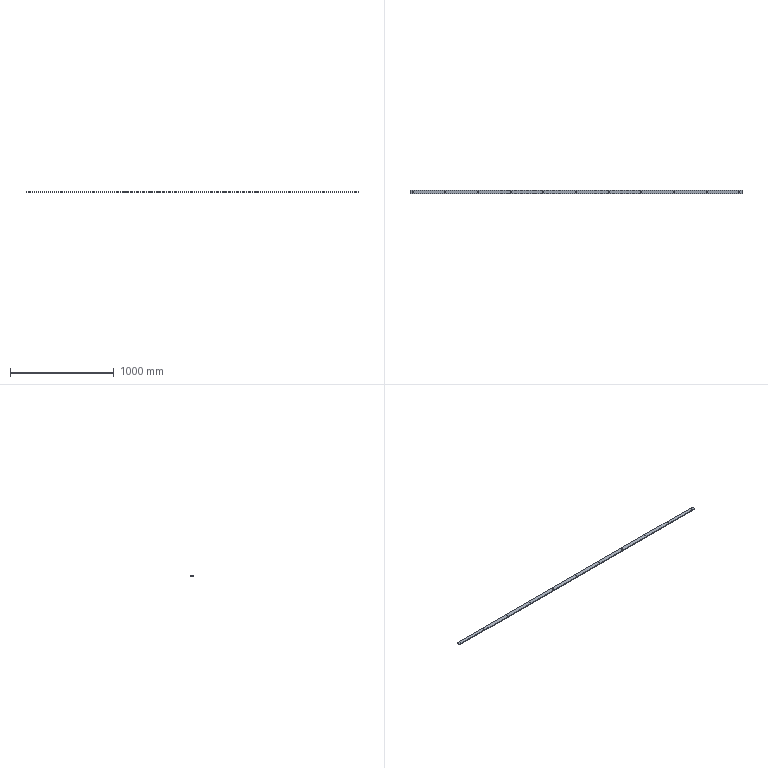Part | SolidWorks | features FlatPattern 1, HoleWzd 1, SMBaseFlange 1, SheetMetal 1 | 1 solid | 28 faces | box 3200 x 35 x 8 mm | volume 891006 mm3 | cylinder 22 | plane 6 | commonest cylinder face diameters 8.5 x22
STEP:
#1=CARTESIAN_POINT('',(-1579.25,0.,-8.));
#2=VERTEX_POINT('',#1);
#3=CARTESIAN_POINT('',(-1570.75,0.,-8.));
#4=VERTEX_POINT('',#3);
#5=CARTESIAN_POINT('',(-1575.,0.,-8.));
#6=DIRECTION('',(0.,0.,1.));
#7=DIRECTION('',(1.,0.,0.));
#8=AXIS2_PLACEMENT_3D('',#5,#6,#7);
#9=CIRCLE('',#8,4.25);
#10=EDGE_CURVE('',#2,#4,#9,.T.);
#11=ORIENTED_EDGE('',*,*,#10,.F.);
#12=CARTESIAN_POINT('',(-1579.25,0.,0.));
#13=VERTEX_POINT('',#12);
#14=CARTESIAN_POINT('',(-1579.25,0.,0.));
#15=DIRECTION('',(0.,0.,1.));
#16=VECTOR('',#15,1000.);
#17=LINE('',#14,#16);
#18=EDGE_CURVE('',#2,#13,#17,.T.);
#19=ORIENTED_EDGE('',*,*,#18,.T.);
#20=CARTESIAN_POINT('',(-1570.75,0.,0.));
#21=VERTEX_POINT('',#20);
#22=CARTESIAN_POINT('',(-1575.,0.,0.));
#23=DIRECTION('',(0.,0.,1.));
#24=DIRECTION('',(1.,0.,0.));
#25=AXIS2_PLACEMENT_3D('',#22,#23,#24);
#26=CIRCLE('',#25,4.25);
#27=EDGE_CURVE('',#13,#21,#26,.T.);
#28=ORIENTED_EDGE('',*,*,#27,.T.);
#29=CARTESIAN_POINT('',(-1570.75,0.,0.));
#30=DIRECTION('',(0.,0.,1.));
#31=VECTOR('',#30,1000.);
#32=LINE('',#29,#31);
#33=EDGE_CURVE('',#4,#21,#32,.T.);
#34=ORIENTED_EDGE('',*,*,#33,.F.);
#35=EDGE_LOOP('',(#11,#19,#28,#34));
#36=FACE_OUTER_BOUND('',#35,.T.);
#37=CARTESIAN_POINT('',(-1575.,0.,0.));
#38=DIRECTION('',(0.,0.,1.));
#39=DIRECTION('',(1.,0.,0.));
#40=AXIS2_PLACEMENT_3D('',#37,#38,#39);
#41=CYLINDRICAL_SURFACE('',#40,4.25);
#42=ADVANCED_FACE('',(#36),#41,.F.);
#43=CARTESIAN_POINT('',(-1264.25,0.,-8.));
#44=VERTEX_POINT('',#43);
#45=CARTESIAN_POINT('',(-1255.75,0.,-8.));
#46=VERTEX_POINT('',#45);
#47=CARTESIAN_POINT('',(-1260.,0.,-8.));
#48=DIRECTION('',(0.,0.,1.));
#49=DIRECTION('',(1.,0.,0.));
#50=AXIS2_PLACEMENT_3D('',#47,#48,#49);
#51=CIRCLE('',#50,4.25);
#52=EDGE_CURVE('',#44,#46,#51,.T.);
#53=ORIENTED_EDGE('',*,*,#52,.F.);
#54=CARTESIAN_POINT('',(-1264.25,0.,0.));
#55=VERTEX_POINT('',#54);
#56=CARTESIAN_POINT('',(-1264.25,0.,0.));
#57=DIRECTION('',(0.,0.,1.));
#58=VECTOR('',#57,1000.);
#59=LINE('',#56,#58);
#60=EDGE_CURVE('',#44,#55,#59,.T.);
#61=ORIENTED_EDGE('',*,*,#60,.T.);
#62=CARTESIAN_POINT('',(-1255.75,0.,0.));
#63=VERTEX_POINT('',#62);
#64=CARTESIAN_POINT('',(-1260.,0.,0.));
#65=DIRECTION('',(0.,0.,1.));
#66=DIRECTION('',(1.,0.,0.));
#67=AXIS2_PLACEMENT_3D('',#64,#65,#66);
#68=CIRCLE('',#67,4.25);
#69=EDGE_CURVE('',#55,#63,#68,.T.);
#70=ORIENTED_EDGE('',*,*,#69,.T.);
#71=CARTESIAN_POINT('',(-1255.75,0.,0.));
#72=DIRECTION('',(0.,0.,1.));
#73=VECTOR('',#72,1000.);
#74=LINE('',#71,#73);
#75=EDGE_CURVE('',#46,#63,#74,.T.);
#76=ORIENTED_EDGE('',*,*,#75,.F.);
#77=EDGE_LOOP('',(#53,#61,#70,#76));
#78=FACE_OUTER_BOUND('',#77,.T.);
#79=CARTESIAN_POINT('',(-1260.,0.,0.));
#80=DIRECTION('',(0.,0.,1.));
#81=DIRECTION('',(1.,0.,0.));
#82=AXIS2_PLACEMENT_3D('',#79,#80,#81);
#83=CYLINDRICAL_SURFACE('',#82,4.25);
#84=ADVANCED_FACE('',(#78),#83,.F.);
#85=CARTESIAN_POINT('',(-949.25,0.,-8.));
#86=VERTEX_POINT('',#85);
#87=CARTESIAN_POINT('',(-940.75,0.,-8.));
#88=VERTEX_POINT('',#87);
#89=CARTESIAN_POINT('',(-945.,0.,-8.));
#90=DIRECTION('',(0.,0.,1.));
#91=DIRECTION('',(1.,0.,0.));
#92=AXIS2_PLACEMENT_3D('',#89,#90,#91);
#93=CIRCLE('',#92,4.25);
#94=EDGE_CURVE('',#86,#88,#93,.T.);
#95=ORIENTED_EDGE('',*,*,#94,.F.);
#96=CARTESIAN_POINT('',(-949.25,0.,0.));
#97=VERTEX_POINT('',#96);
#98=CARTESIAN_POINT('',(-949.25,0.,0.));
#99=DIRECTION('',(0.,0.,1.));
#100=VECTOR('',#99,1000.);
#101=LINE('',#98,#100);
#102=EDGE_CURVE('',#86,#97,#101,.T.);
#103=ORIENTED_EDGE('',*,*,#102,.T.);
#104=CARTESIAN_POINT('',(-940.75,0.,0.));
#105=VERTEX_POINT('',#104);
#106=CARTESIAN_POINT('',(-945.,0.,0.));
#107=DIRECTION('',(0.,0.,1.));
#108=DIRECTION('',(1.,0.,0.));
#109=AXIS2_PLACEMENT_3D('',#106,#107,#108);
#110=CIRCLE('',#109,4.25);
#111=EDGE_CURVE('',#97,#105,#110,.T.);
#112=ORIENTED_EDGE('',*,*,#111,.T.);
#113=CARTESIAN_POINT('',(-940.75,0.,0.));
#114=DIRECTION('',(0.,0.,1.));
#115=VECTOR('',#114,1000.);
#116=LINE('',#113,#115);
#117=EDGE_CURVE('',#88,#105,#116,.T.);
#118=ORIENTED_EDGE('',*,*,#117,.F.);
#119=EDGE_LOOP('',(#95,#103,#112,#118));
#120=FACE_OUTER_BOUND('',#119,.T.);
#121=CARTESIAN_POINT('',(-945.,0.,0.));
#122=DIRECTION('',(0.,0.,1.));
#123=DIRECTION('',(1.,0.,0.));
#124=AXIS2_PLACEMENT_3D('',#121,#122,#123);
#125=CYLINDRICAL_SURFACE('',#124,4.25);
#126=ADVANCED_FACE('',(#120),#125,.F.);
#127=CARTESIAN_POINT('',(-634.25,0.,-8.));
#128=VERTEX_POINT('',#127);
#129=CARTESIAN_POINT('',(-625.75,0.,-8.));
#130=VERTEX_POINT('',#129);
#131=CARTESIAN_POINT('',(-630.,0.,-8.));
#132=DIRECTION('',(0.,0.,1.));
#133=DIRECTION('',(1.,0.,0.));
#134=AXIS2_PLACEMENT_3D('',#131,#132,#133);
#135=CIRCLE('',#134,4.25);
#136=EDGE_CURVE('',#128,#130,#135,.T.);
#137=ORIENTED_EDGE('',*,*,#136,.F.);
#138=CARTESIAN_POINT('',(-634.25,0.,0.));
#139=VERTEX_POINT('',#138);
#140=CARTESIAN_POINT('',(-634.25,0.,0.));
#141=DIRECTION('',(0.,0.,1.));
#142=VECTOR('',#141,1000.);
#143=LINE('',#140,#142);
#144=EDGE_CURVE('',#128,#139,#143,.T.);
#145=ORIENTED_EDGE('',*,*,#144,.T.);
#146=CARTESIAN_POINT('',(-625.75,0.,0.));
#147=VERTEX_POINT('',#146);
#148=CARTESIAN_POINT('',(-630.,0.,0.));
#149=DIRECTION('',(0.,0.,1.));
#150=DIRECTION('',(1.,0.,0.));
#151=AXIS2_PLACEMENT_3D('',#148,#149,#150);
#152=CIRCLE('',#151,4.25);
#153=EDGE_CURVE('',#139,#147,#152,.T.);
#154=ORIENTED_EDGE('',*,*,#153,.T.);
#155=CARTESIAN_POINT('',(-625.75,0.,0.));
#156=DIRECTION('',(0.,0.,1.));
#157=VECTOR('',#156,1000.);
#158=LINE('',#155,#157);
#159=EDGE_CURVE('',#130,#147,#158,.T.);
#160=ORIENTED_EDGE('',*,*,#159,.F.);
#161=EDGE_LOOP('',(#137,#145,#154,#160));
#162=FACE_OUTER_BOUND('',#161,.T.);
#163=CARTESIAN_POINT('',(-630.,0.,0.));
#164=DIRECTION('',(0.,0.,1.));
#165=DIRECTION('',(1.,0.,0.));
#166=AXIS2_PLACEMENT_3D('',#163,#164,#165);
#167=CYLINDRICAL_SURFACE('',#166,4.25);
#168=ADVANCED_FACE('',(#162),#167,.F.);
#169=CARTESIAN_POINT('',(-319.25,0.,-8.));
#170=VERTEX_POINT('',#169);
#171=CARTESIAN_POINT('',(-310.75,0.,-8.));
#172=VERTEX_POINT('',#171);
#173=CARTESIAN_POINT('',(-315.,0.,-8.));
#174=DIRECTION('',(0.,0.,1.));
#175=DIRECTION('',(1.,0.,0.));
#176=AXIS2_PLACEMENT_3D('',#173,#174,#175);
#177=CIRCLE('',#176,4.25);
#178=EDGE_CURVE('',#170,#172,#177,.T.);
#179=ORIENTED_EDGE('',*,*,#178,.F.);
#180=CARTESIAN_POINT('',(-319.25,0.,0.));
#181=VERTEX_POINT('',#180);
#182=CARTESIAN_POINT('',(-319.25,0.,0.));
#183=DIRECTION('',(0.,0.,1.));
#184=VECTOR('',#183,1000.);
#185=LINE('',#182,#184);
#186=EDGE_CURVE('',#170,#181,#185,.T.);
#187=ORIENTED_EDGE('',*,*,#186,.T.);
#188=CARTESIAN_POINT('',(-310.75,0.,0.));
#189=VERTEX_POINT('',#188);
#190=CARTESIAN_POINT('',(-315.,0.,0.));
#191=DIRECTION('',(0.,0.,1.));
#192=DIRECTION('',(1.,0.,0.));
#193=AXIS2_PLACEMENT_3D('',#190,#191,#192);
#194=CIRCLE('',#193,4.25);
#195=EDGE_CURVE('',#181,#189,#194,.T.);
#196=ORIENTED_EDGE('',*,*,#195,.T.);
#197=CARTESIAN_POINT('',(-310.75,0.,0.));
#198=DIRECTION('',(0.,0.,1.));
#199=VECTOR('',#198,1000.);
#200=LINE('',#197,#199);
#201=EDGE_CURVE('',#172,#189,#200,.T.);
#202=ORIENTED_EDGE('',*,*,#201,.F.);
#203=EDGE_LOOP('',(#179,#187,#196,#202));
#204=FACE_OUTER_BOUND('',#203,.T.);
#205=CARTESIAN_POINT('',(-315.,0.,0.));
#206=DIRECTION('',(0.,0.,1.));
#207=DIRECTION('',(1.,0.,0.));
#208=AXIS2_PLACEMENT_3D('',#205,#206,#207);
#209=CYLINDRICAL_SURFACE('',#208,4.25);
#210=ADVANCED_FACE('',(#204),#209,.F.);
#211=CARTESIAN_POINT('',(-4.25,0.,-8.));
#212=VERTEX_POINT('',#211);
#213=CARTESIAN_POINT('',(4.25,0.,-8.));
#214=VERTEX_POINT('',#213);
#215=CARTESIAN_POINT('',(0.,0.,-8.));
#216=DIRECTION('',(0.,0.,1.));
#217=DIRECTION('',(1.,0.,0.));
#218=AXIS2_PLACEMENT_3D('',#215,#216,#217);
#219=CIRCLE('',#218,4.25);
#220=EDGE_CURVE('',#212,#214,#219,.T.);
#221=ORIENTED_EDGE('',*,*,#220,.F.);
#222=CARTESIAN_POINT('',(-4.25,0.,0.));
#223=VERTEX_POINT('',#222);
#224=CARTESIAN_POINT('',(-4.25,0.,0.));
#225=DIRECTION('',(0.,0.,1.));
#226=VECTOR('',#225,1000.);
#227=LINE('',#224,#226);
#228=EDGE_CURVE('',#212,#223,#227,.T.);
#229=ORIENTED_EDGE('',*,*,#228,.T.);
#230=CARTESIAN_POINT('',(4.25,0.,0.));
#231=VERTEX_POINT('',#230);
#232=CARTESIAN_POINT('',(0.,0.,0.));
#233=DIRECTION('',(0.,0.,1.));
#234=DIRECTION('',(1.,0.,0.));
#235=AXIS2_PLACEMENT_3D('',#232,#233,#234);
#236=CIRCLE('',#235,4.25);
#237=EDGE_CURVE('',#223,#231,#236,.T.);
#238=ORIENTED_EDGE('',*,*,#237,.T.);
#239=CARTESIAN_POINT('',(4.25,0.,0.));
#240=DIRECTION('',(0.,0.,1.));
#241=VECTOR('',#240,1000.);
#242=LINE('',#239,#241);
#243=EDGE_CURVE('',#214,#231,#242,.T.);
#244=ORIENTED_EDGE('',*,*,#243,.F.);
#245=EDGE_LOOP('',(#221,#229,#238,#244));
#246=FACE_OUTER_BOUND('',#245,.T.);
#247=CARTESIAN_POINT('',(0.,0.,0.));
#248=DIRECTION('',(0.,0.,1.));
#249=DIRECTION('',(1.,0.,0.));
#250=AXIS2_PLACEMENT_3D('',#247,#248,#249);
#251=CYLINDRICAL_SURFACE('',#250,4.25);
#252=ADVANCED_FACE('',(#246),#251,.F.);
#253=CARTESIAN_POINT('',(310.75,0.,-8.));
#254=VERTEX_POINT('',#253);
#255=CARTESIAN_POINT('',(319.25,0.,-8.));
#256=VERTEX_POINT('',#255);
#257=CARTESIAN_POINT('',(315.,0.,-8.));
#258=DIRECTION('',(0.,0.,1.));
#259=DIRECTION('',(1.,0.,0.));
#260=AXIS2_PLACEMENT_3D('',#257,#258,#259);
#261=CIRCLE('',#260,4.25);
#262=EDGE_CURVE('',#254,#256,#261,.T.);
#263=ORIENTED_EDGE('',*,*,#262,.F.);
#264=CARTESIAN_POINT('',(310.75,0.,0.));
#265=VERTEX_POINT('',#264);
#266=CARTESIAN_POINT('',(310.75,0.,0.));
#267=DIRECTION('',(0.,0.,1.));
#268=VECTOR('',#267,1000.);
#269=LINE('',#266,#268);
#270=EDGE_CURVE('',#254,#265,#269,.T.);
#271=ORIENTED_EDGE('',*,*,#270,.T.);
#272=CARTESIAN_POINT('',(319.25,0.,0.));
#273=VERTEX_POINT('',#272);
#274=CARTESIAN_POINT('',(315.,0.,0.));
#275=DIRECTION('',(0.,0.,1.));
#276=DIRECTION('',(1.,0.,0.));
#277=AXIS2_PLACEMENT_3D('',#274,#275,#276);
#278=CIRCLE('',#277,4.25);
#279=EDGE_CURVE('',#265,#273,#278,.T.);
#280=ORIENTED_EDGE('',*,*,#279,.T.);
#281=CARTESIAN_POINT('',(319.25,0.,0.));
#282=DIRECTION('',(0.,0.,1.));
#283=VECTOR('',#282,1000.);
#284=LINE('',#281,#283);
#285=EDGE_CURVE('',#256,#273,#284,.T.);
#286=ORIENTED_EDGE('',*,*,#285,.F.);
#287=EDGE_LOOP('',(#263,#271,#280,#286));
#288=FACE_OUTER_BOUND('',#287,.T.);
#289=CARTESIAN_POINT('',(315.,0.,0.));
#290=DIRECTION('',(0.,0.,1.));
#291=DIRECTION('',(1.,0.,0.));
#292=AXIS2_PLACEMENT_3D('',#289,#290,#291);
#293=CYLINDRICAL_SURFACE('',#292,4.25);
#294=ADVANCED_FACE('',(#288),#293,.F.);
#295=CARTESIAN_POINT('',(625.75,0.,-8.));
#296=VERTEX_POINT('',#295);
#297=CARTESIAN_POINT('',(634.25,0.,-8.));
#298=VERTEX_POINT('',#297);
#299=CARTESIAN_POINT('',(630.,0.,-8.));
#300=DIRECTION('',(0.,0.,1.));
#301=DIRECTION('',(1.,0.,0.));
#302=AXIS2_PLACEMENT_3D('',#299,#300,#301);
#303=CIRCLE('',#302,4.25);
#304=EDGE_CURVE('',#296,#298,#303,.T.);
#305=ORIENTED_EDGE('',*,*,#304,.F.);
#306=CARTESIAN_POINT('',(625.75,0.,0.));
#307=VERTEX_POINT('',#306);
#308=CARTESIAN_POINT('',(625.75,0.,0.));
#309=DIRECTION('',(0.,0.,1.));
#310=VECTOR('',#309,1000.);
#311=LINE('',#308,#310);
#312=EDGE_CURVE('',#296,#307,#311,.T.);
#313=ORIENTED_EDGE('',*,*,#312,.T.);
#314=CARTESIAN_POINT('',(634.25,0.,0.));
#315=VERTEX_POINT('',#314);
#316=CARTESIAN_POINT('',(630.,0.,0.));
#317=DIRECTION('',(0.,0.,1.));
#318=DIRECTION('',(1.,0.,0.));
#319=AXIS2_PLACEMENT_3D('',#316,#317,#318);
#320=CIRCLE('',#319,4.25);
#321=EDGE_CURVE('',#307,#315,#320,.T.);
#322=ORIENTED_EDGE('',*,*,#321,.T.);
#323=CARTESIAN_POINT('',(634.25,0.,0.));
#324=DIRECTION('',(0.,0.,1.));
#325=VECTOR('',#324,1000.);
#326=LINE('',#323,#325);
#327=EDGE_CURVE('',#298,#315,#326,.T.);
#328=ORIENTED_EDGE('',*,*,#327,.F.);
#329=EDGE_LOOP('',(#305,#313,#322,#328));
#330=FACE_OUTER_BOUND('',#329,.T.);
#331=CARTESIAN_POINT('',(630.,0.,0.));
#332=DIRECTION('',(0.,0.,1.));
#333=DIRECTION('',(1.,0.,0.));
#334=AXIS2_PLACEMENT_3D('',#331,#332,#333);
#335=CYLINDRICAL_SURFACE('',#334,4.25);
#336=ADVANCED_FACE('',(#330),#335,.F.);
#337=CARTESIAN_POINT('',(940.75,0.,-8.));
#338=VERTEX_POINT('',#337);
#339=CARTESIAN_POINT('',(949.25,0.,-8.));
#340=VERTEX_POINT('',#339);
#341=CARTESIAN_POINT('',(945.,0.,-8.));
#342=DIRECTION('',(0.,0.,1.));
#343=DIRECTION('',(1.,0.,0.));
#344=AXIS2_PLACEMENT_3D('',#341,#342,#343);
#345=CIRCLE('',#344,4.25);
#346=EDGE_CURVE('',#338,#340,#345,.T.);
#347=ORIENTED_EDGE('',*,*,#346,.F.);
#348=CARTESIAN_POINT('',(940.75,0.,0.));
#349=VERTEX_POINT('',#348);
#350=CARTESIAN_POINT('',(940.75,0.,0.));
#351=DIRECTION('',(0.,0.,1.));
#352=VECTOR('',#351,1000.);
#353=LINE('',#350,#352);
#354=EDGE_CURVE('',#338,#349,#353,.T.);
#355=ORIENTED_EDGE('',*,*,#354,.T.);
#356=CARTESIAN_POINT('',(949.25,0.,0.));
#357=VERTEX_POINT('',#356);
#358=CARTESIAN_POINT('',(945.,0.,0.));
#359=DIRECTION('',(0.,0.,1.));
#360=DIRECTION('',(1.,0.,0.));
#361=AXIS2_PLACEMENT_3D('',#358,#359,#360);
#362=CIRCLE('',#361,4.25);
#363=EDGE_CURVE('',#349,#357,#362,.T.);
#364=ORIENTED_EDGE('',*,*,#363,.T.);
#365=CARTESIAN_POINT('',(949.25,0.,0.));
#366=DIRECTION('',(0.,0.,1.));
#367=VECTOR('',#366,1000.);
#368=LINE('',#365,#367);
#369=EDGE_CURVE('',#340,#357,#368,.T.);
#370=ORIENTED_EDGE('',*,*,#369,.F.);
#371=EDGE_LOOP('',(#347,#355,#364,#370));
#372=FACE_OUTER_BOUND('',#371,.T.);
#373=CARTESIAN_POINT('',(945.,0.,0.));
#374=DIRECTION('',(0.,0.,1.));
#375=DIRECTION('',(1.,0.,0.));
#376=AXIS2_PLACEMENT_3D('',#373,#374,#375);
#377=CYLINDRICAL_SURFACE('',#376,4.25);
#378=ADVANCED_FACE('',(#372),#377,.F.);
#379=CARTESIAN_POINT('',(1255.75,0.,-8.));
#380=VERTEX_POINT('',#379);
#381=CARTESIAN_POINT('',(1264.25,0.,-8.));
#382=VERTEX_POINT('',#381);
#383=CARTESIAN_POINT('',(1260.,0.,-8.));
#384=DIRECTION('',(0.,0.,1.));
#385=DIRECTION('',(1.,0.,0.));
#386=AXIS2_PLACEMENT_3D('',#383,#384,#385);
#387=CIRCLE('',#386,4.25);
#388=EDGE_CURVE('',#380,#382,#387,.T.);
#389=ORIENTED_EDGE('',*,*,#388,.F.);
#390=CARTESIAN_POINT('',(1255.75,0.,0.));
#391=VERTEX_POINT('',#390);
#392=CARTESIAN_POINT('',(1255.75,0.,0.));
#393=DIRECTION('',(0.,0.,1.));
#394=VECTOR('',#393,1000.);
#395=LINE('',#392,#394);
#396=EDGE_CURVE('',#380,#391,#395,.T.);
#397=ORIENTED_EDGE('',*,*,#396,.T.);
#398=CARTESIAN_POINT('',(1264.25,0.,0.));
#399=VERTEX_POINT('',#398);
#400=CARTESIAN_POINT('',(1260.,0.,0.));
#401=DIRECTION('',(0.,0.,1.));
#402=DIRECTION('',(1.,0.,0.));
#403=AXIS2_PLACEMENT_3D('',#400,#401,#402);
#404=CIRCLE('',#403,4.25);
#405=EDGE_CURVE('',#391,#399,#404,.T.);
#406=ORIENTED_EDGE('',*,*,#405,.T.);
#407=CARTESIAN_POINT('',(1264.25,0.,0.));
#408=DIRECTION('',(0.,0.,1.));
#409=VECTOR('',#408,1000.);
#410=LINE('',#407,#409);
#411=EDGE_CURVE('',#382,#399,#410,.T.);
#412=ORIENTED_EDGE('',*,*,#411,.F.);
#413=EDGE_LOOP('',(#389,#397,#406,#412));
#414=FACE_OUTER_BOUND('',#413,.T.);
#415=CARTESIAN_POINT('',(1260.,0.,0.));
#416=DIRECTION('',(0.,0.,1.));
#417=DIRECTION('',(1.,0.,0.));
#418=AXIS2_PLACEMENT_3D('',#415,#416,#417);
#419=CYLINDRICAL_SURFACE('',#418,4.25);
#420=ADVANCED_FACE('',(#414),#419,.F.);
#421=CARTESIAN_POINT('',(1570.75,0.,-8.));
#422=VERTEX_POINT('',#421);
#423=CARTESIAN_POINT('',(1579.25,0.,-8.));
#424=VERTEX_POINT('',#423);
#425=CARTESIAN_POINT('',(1575.,0.,-8.));
#426=DIRECTION('',(0.,0.,1.));
#427=DIRECTION('',(1.,0.,0.));
#428=AXIS2_PLACEMENT_3D('',#425,#426,#427);
#429=CIRCLE('',#428,4.25);
#430=EDGE_CURVE('',#422,#424,#429,.T.);
#431=ORIENTED_EDGE('',*,*,#430,.F.);
#432=CARTESIAN_POINT('',(1570.75,0.,0.));
#433=VERTEX_POINT('',#432);
#434=CARTESIAN_POINT('',(1570.75,0.,0.));
#435=DIRECTION('',(0.,0.,1.));
#436=VECTOR('',#435,1000.);
#437=LINE('',#434,#436);
#438=EDGE_CURVE('',#422,#433,#437,.T.);
#439=ORIENTED_EDGE('',*,*,#438,.T.);
#440=CARTESIAN_POINT('',(1579.25,0.,0.));
#441=VERTEX_POINT('',#440);
#442=CARTESIAN_POINT('',(1575.,0.,0.));
#443=DIRECTION('',(0.,0.,1.));
#444=DIRECTION('',(1.,0.,0.));
#445=AXIS2_PLACEMENT_3D('',#442,#443,#444);
#446=CIRCLE('',#445,4.25);
#447=EDGE_CURVE('',#433,#441,#446,.T.);
#448=ORIENTED_EDGE('',*,*,#447,.T.);
#449=CARTESIAN_POINT('',(1579.25,0.,0.));
#450=DIRECTION('',(0.,0.,1.));
#451=VECTOR('',#450,1000.);
#452=LINE('',#449,#451);
#453=EDGE_CURVE('',#424,#441,#452,.T.);
#454=ORIENTED_EDGE('',*,*,#453,.F.);
#455=EDGE_LOOP('',(#431,#439,#448,#454));
#456=FACE_OUTER_BOUND('',#455,.T.);
#457=CARTESIAN_POINT('',(1575.,0.,0.));
#458=DIRECTION('',(0.,0.,1.));
#459=DIRECTION('',(1.,0.,0.));
#460=AXIS2_PLACEMENT_3D('',#457,#458,#459);
#461=CYLINDRICAL_SURFACE('',#460,4.25);
#462=ADVANCED_FACE('',(#456),#461,.F.);
#463=CARTESIAN_POINT('',(1600.,-17.5,0.));
#464=VERTEX_POINT('',#463);
#465=CARTESIAN_POINT('',(1600.,17.5,0.));
#466=VERTEX_POINT('',#465);
#467=CARTESIAN_POINT('',(1600.,17.5,0.));
#468=DIRECTION('',(0.,1.,0.));
#469=VECTOR('',#468,1000.);
#470=LINE('',#467,#469);
#471=EDGE_CURVE('',#464,#466,#470,.T.);
#472=ORIENTED_EDGE('',*,*,#471,.F.);
#473=CARTESIAN_POINT('',(1600.,-17.5,-8.));
#474=VERTEX_POINT('',#473);
#475=CARTESIAN_POINT('',(1600.,-17.5,-8.));
#476=DIRECTION('',(0.,0.,1.));
#477=VECTOR('',#476,1000.);
#478=LINE('',#475,#477);
#479=EDGE_CURVE('',#474,#464,#478,.T.);
#480=ORIENTED_EDGE('',*,*,#479,.F.);
#481=CARTESIAN_POINT('',(1600.,17.5,-8.));
#482=VERTEX_POINT('',#481);
#483=CARTESIAN_POINT('',(1600.,17.5,-8.));
#484=DIRECTION('',(0.,1.,0.));
#485=VECTOR('',#484,1000.);
#486=LINE('',#483,#485);
#487=EDGE_CURVE('',#474,#482,#486,.T.);
#488=ORIENTED_EDGE('',*,*,#487,.T.);
#489=CARTESIAN_POINT('',(1600.,17.5,-8.));
#490=DIRECTION('',(0.,0.,1.));
#491=VECTOR('',#490,1000.);
#492=LINE('',#489,#491);
#493=EDGE_CURVE('',#482,#466,#492,.T.);
#494=ORIENTED_EDGE('',*,*,#493,.T.);
#495=EDGE_LOOP('',(#472,#480,#488,#494));
#496=FACE_OUTER_BOUND('',#495,.T.);
#497=CARTESIAN_POINT('',(1600.,17.5,-8.));
#498=DIRECTION('',(1.,0.,0.));
#499=DIRECTION('',(0.,0.,-1.));
#500=AXIS2_PLACEMENT_3D('',#497,#498,#499);
#501=PLANE('',#500);
#502=ADVANCED_FACE('',(#496),#501,.T.);
#503=CARTESIAN_POINT('',(-1600.,-17.5,0.));
#504=VERTEX_POINT('',#503);
#505=CARTESIAN_POINT('',(-1600.,-17.5,0.));
#506=DIRECTION('',(1.,0.,0.));
#507=VECTOR('',#506,1000.);
#508=LINE('',#505,#507);
#509=EDGE_CURVE('',#504,#464,#508,.T.);
#510=ORIENTED_EDGE('',*,*,#509,.F.);
#511=CARTESIAN_POINT('',(-1600.,-17.5,-8.));
#512=VERTEX_POINT('',#511);
#513=CARTESIAN_POINT('',(-1600.,-17.5,-8.));
#514=DIRECTION('',(0.,0.,1.));
#515=VECTOR('',#514,1000.);
#516=LINE('',#513,#515);
#517=EDGE_CURVE('',#512,#504,#516,.T.);
#518=ORIENTED_EDGE('',*,*,#517,.F.);
#519=CARTESIAN_POINT('',(-1600.,-17.5,-8.));
#520=DIRECTION('',(1.,0.,0.));
#521=VECTOR('',#520,1000.);
#522=LINE('',#519,#521);
#523=EDGE_CURVE('',#512,#474,#522,.T.);
#524=ORIENTED_EDGE('',*,*,#523,.T.);
#525=ORIENTED_EDGE('',*,*,#479,.T.);
#526=EDGE_LOOP('',(#510,#518,#524,#525));
#527=FACE_OUTER_BOUND('',#526,.T.);
#528=CARTESIAN_POINT('',(-1600.,-17.5,-8.));
#529=DIRECTION('',(0.,-1.,0.));
#530=DIRECTION('',(0.,0.,-1.));
#531=AXIS2_PLACEMENT_3D('',#528,#529,#530);
#532=PLANE('',#531);
#533=ADVANCED_FACE('',(#527),#532,.T.);
#534=CARTESIAN_POINT('',(-1600.,17.5,0.));
#535=VERTEX_POINT('',#534);
#536=CARTESIAN_POINT('',(-1600.,17.5,0.));
#537=DIRECTION('',(0.,-1.,0.));
#538=VECTOR('',#537,1000.);
#539=LINE('',#536,#538);
#540=EDGE_CURVE('',#535,#504,#539,.T.);
#541=ORIENTED_EDGE('',*,*,#540,.F.);
#542=CARTESIAN_POINT('',(-1600.,17.5,-8.));
#543=VERTEX_POINT('',#542);
#544=CARTESIAN_POINT('',(-1600.,17.5,-8.));
#545=DIRECTION('',(0.,0.,1.));
#546=VECTOR('',#545,1000.);
#547=LINE('',#544,#546);
#548=EDGE_CURVE('',#543,#535,#547,.T.);
#549=ORIENTED_EDGE('',*,*,#548,.F.);
#550=CARTESIAN_POINT('',(-1600.,17.5,-8.));
#551=DIRECTION('',(0.,-1.,0.));
#552=VECTOR('',#551,1000.);
#553=LINE('',#550,#552);
#554=EDGE_CURVE('',#543,#512,#553,.T.);
#555=ORIENTED_EDGE('',*,*,#554,.T.);
#556=ORIENTED_EDGE('',*,*,#517,.T.);
#557=EDGE_LOOP('',(#541,#549,#555,#556));
#558=FACE_OUTER_BOUND('',#557,.T.);
#559=CARTESIAN_POINT('',(-1600.,17.5,-8.));
#560=DIRECTION('',(-1.,0.,0.));
#561=DIRECTION('',(0.,0.,1.));
#562=AXIS2_PLACEMENT_3D('',#559,#560,#561);
#563=PLANE('',#562);
#564=ADVANCED_FACE('',(#558),#563,.T.);
#565=CARTESIAN_POINT('',(-1600.,17.5,0.));
#566=DIRECTION('',(-1.,0.,0.));
#567=VECTOR('',#566,1000.);
#568=LINE('',#565,#567);
#569=EDGE_CURVE('',#466,#535,#568,.T.);
#570=ORIENTED_EDGE('',*,*,#569,.F.);
#571=ORIENTED_EDGE('',*,*,#493,.F.);
#572=CARTESIAN_POINT('',(-1600.,17.5,-8.));
#573=DIRECTION('',(-1.,0.,0.));
#574=VECTOR('',#573,1000.);
#575=LINE('',#572,#574);
#576=EDGE_CURVE('',#482,#543,#575,.T.);
#577=ORIENTED_EDGE('',*,*,#576,.T.);
#578=ORIENTED_EDGE('',*,*,#548,.T.);
#579=EDGE_LOOP('',(#570,#571,#577,#578));
#580=FACE_OUTER_BOUND('',#579,.T.);
#581=CARTESIAN_POINT('',(-1600.,17.5,-8.));
#582=DIRECTION('',(0.,1.,0.));
#583=DIRECTION('',(0.,0.,1.));
#584=AXIS2_PLACEMENT_3D('',#581,#582,#583);
#585=PLANE('',#584);
#586=ADVANCED_FACE('',(#580),#585,.T.);
#587=CARTESIAN_POINT('',(-1575.,0.,-8.));
#588=DIRECTION('',(0.,0.,1.));
#589=DIRECTION('',(1.,0.,0.));
#590=AXIS2_PLACEMENT_3D('',#587,#588,#589);
#591=CIRCLE('',#590,4.25);
#592=EDGE_CURVE('',#4,#2,#591,.T.);
#593=ORIENTED_EDGE('',*,*,#592,.T.);
#594=ORIENTED_EDGE('',*,*,#10,.T.);
#595=EDGE_LOOP('',(#593,#594));
#596=FACE_BOUND('',#595,.T.);
#597=CARTESIAN_POINT('',(-1260.,0.,-8.));
#598=DIRECTION('',(0.,0.,1.));
#599=DIRECTION('',(1.,0.,0.));
#600=AXIS2_PLACEMENT_3D('',#597,#598,#599);
#601=CIRCLE('',#600,4.25);
#602=EDGE_CURVE('',#46,#44,#601,.T.);
#603=ORIENTED_EDGE('',*,*,#602,.T.);
#604=ORIENTED_EDGE('',*,*,#52,.T.);
#605=EDGE_LOOP('',(#603,#604));
#606=FACE_BOUND('',#605,.T.);
#607=CARTESIAN_POINT('',(-945.,0.,-8.));
#608=DIRECTION('',(0.,0.,1.));
#609=DIRECTION('',(1.,0.,0.));
#610=AXIS2_PLACEMENT_3D('',#607,#608,#609);
#611=CIRCLE('',#610,4.25);
#612=EDGE_CURVE('',#88,#86,#611,.T.);
#613=ORIENTED_EDGE('',*,*,#612,.T.);
#614=ORIENTED_EDGE('',*,*,#94,.T.);
#615=EDGE_LOOP('',(#613,#614));
#616=FACE_BOUND('',#615,.T.);
#617=CARTESIAN_POINT('',(-630.,0.,-8.));
#618=DIRECTION('',(0.,0.,1.));
#619=DIRECTION('',(1.,0.,0.));
#620=AXIS2_PLACEMENT_3D('',#617,#618,#619);
#621=CIRCLE('',#620,4.25);
#622=EDGE_CURVE('',#130,#128,#621,.T.);
#623=ORIENTED_EDGE('',*,*,#622,.T.);
#624=ORIENTED_EDGE('',*,*,#136,.T.);
#625=EDGE_LOOP('',(#623,#624));
#626=FACE_BOUND('',#625,.T.);
#627=CARTESIAN_POINT('',(-315.,0.,-8.));
#628=DIRECTION('',(0.,0.,1.));
#629=DIRECTION('',(1.,0.,0.));
#630=AXIS2_PLACEMENT_3D('',#627,#628,#629);
#631=CIRCLE('',#630,4.25);
#632=EDGE_CURVE('',#172,#170,#631,.T.);
#633=ORIENTED_EDGE('',*,*,#632,.T.);
#634=ORIENTED_EDGE('',*,*,#178,.T.);
#635=EDGE_LOOP('',(#633,#634));
#636=FACE_BOUND('',#635,.T.);
#637=CARTESIAN_POINT('',(0.,0.,-8.));
#638=DIRECTION('',(0.,0.,1.));
#639=DIRECTION('',(1.,0.,0.));
#640=AXIS2_PLACEMENT_3D('',#637,#638,#639);
#641=CIRCLE('',#640,4.25);
#642=EDGE_CURVE('',#214,#212,#641,.T.);
#643=ORIENTED_EDGE('',*,*,#642,.T.);
#644=ORIENTED_EDGE('',*,*,#220,.T.);
#645=EDGE_LOOP('',(#643,#644));
#646=FACE_BOUND('',#645,.T.);
#647=CARTESIAN_POINT('',(315.,0.,-8.));
#648=DIRECTION('',(0.,0.,1.));
#649=DIRECTION('',(1.,0.,0.));
#650=AXIS2_PLACEMENT_3D('',#647,#648,#649);
#651=CIRCLE('',#650,4.25);
#652=EDGE_CURVE('',#256,#254,#651,.T.);
#653=ORIENTED_EDGE('',*,*,#652,.T.);
#654=ORIENTED_EDGE('',*,*,#262,.T.);
#655=EDGE_LOOP('',(#653,#654));
#656=FACE_BOUND('',#655,.T.);
#657=CARTESIAN_POINT('',(630.,0.,-8.));
#658=DIRECTION('',(0.,0.,1.));
#659=DIRECTION('',(1.,0.,0.));
#660=AXIS2_PLACEMENT_3D('',#657,#658,#659);
#661=CIRCLE('',#660,4.25);
#662=EDGE_CURVE('',#298,#296,#661,.T.);
#663=ORIENTED_EDGE('',*,*,#662,.T.);
#664=ORIENTED_EDGE('',*,*,#304,.T.);
#665=EDGE_LOOP('',(#663,#664));
#666=FACE_BOUND('',#665,.T.);
#667=CARTESIAN_POINT('',(945.,0.,-8.));
#668=DIRECTION('',(0.,0.,1.));
#669=DIRECTION('',(1.,0.,0.));
#670=AXIS2_PLACEMENT_3D('',#667,#668,#669);
#671=CIRCLE('',#670,4.25);
#672=EDGE_CURVE('',#340,#338,#671,.T.);
#673=ORIENTED_EDGE('',*,*,#672,.T.);
#674=ORIENTED_EDGE('',*,*,#346,.T.);
#675=EDGE_LOOP('',(#673,#674));
#676=FACE_BOUND('',#675,.T.);
#677=CARTESIAN_POINT('',(1260.,0.,-8.));
#678=DIRECTION('',(0.,0.,1.));
#679=DIRECTION('',(1.,0.,0.));
#680=AXIS2_PLACEMENT_3D('',#677,#678,#679);
#681=CIRCLE('',#680,4.25);
#682=EDGE_CURVE('',#382,#380,#681,.T.);
#683=ORIENTED_EDGE('',*,*,#682,.T.);
#684=ORIENTED_EDGE('',*,*,#388,.T.);
#685=EDGE_LOOP('',(#683,#684));
#686=FACE_BOUND('',#685,.T.);
#687=CARTESIAN_POINT('',(1575.,0.,-8.));
#688=DIRECTION('',(0.,0.,1.));
#689=DIRECTION('',(1.,0.,0.));
#690=AXIS2_PLACEMENT_3D('',#687,#688,#689);
#691=CIRCLE('',#690,4.25);
#692=EDGE_CURVE('',#424,#422,#691,.T.);
#693=ORIENTED_EDGE('',*,*,#692,.T.);
#694=ORIENTED_EDGE('',*,*,#430,.T.);
#695=EDGE_LOOP('',(#693,#694));
#696=FACE_BOUND('',#695,.T.);
#697=ORIENTED_EDGE('',*,*,#487,.F.);
#698=ORIENTED_EDGE('',*,*,#523,.F.);
#699=ORIENTED_EDGE('',*,*,#554,.F.);
#700=ORIENTED_EDGE('',*,*,#576,.F.);
#701=EDGE_LOOP('',(#697,#698,#699,#700));
#702=FACE_OUTER_BOUND('',#701,.T.);
#703=CARTESIAN_POINT('',(0.,0.,-8.));
#704=DIRECTION('',(0.,0.,1.));
#705=DIRECTION('',(1.,0.,0.));
#706=AXIS2_PLACEMENT_3D('',#703,#704,#705);
#707=PLANE('',#706);
#708=ADVANCED_FACE('',(#596,#606,#616,#626,#636,#646,#656,#666,#676,#686,#696,#702),#707,.F.);
#709=CARTESIAN_POINT('',(-1575.,0.,0.));
#710=DIRECTION('',(0.,0.,1.));
#711=DIRECTION('',(1.,0.,0.));
#712=AXIS2_PLACEMENT_3D('',#709,#710,#711);
#713=CIRCLE('',#712,4.25);
#714=EDGE_CURVE('',#21,#13,#713,.T.);
#715=ORIENTED_EDGE('',*,*,#714,.F.);
#716=ORIENTED_EDGE('',*,*,#27,.F.);
#717=EDGE_LOOP('',(#715,#716));
#718=FACE_BOUND('',#717,.T.);
#719=CARTESIAN_POINT('',(-1260.,0.,0.));
#720=DIRECTION('',(0.,0.,1.));
#721=DIRECTION('',(1.,0.,0.));
#722=AXIS2_PLACEMENT_3D('',#719,#720,#721);
#723=CIRCLE('',#722,4.25);
#724=EDGE_CURVE('',#63,#55,#723,.T.);
#725=ORIENTED_EDGE('',*,*,#724,.F.);
#726=ORIENTED_EDGE('',*,*,#69,.F.);
#727=EDGE_LOOP('',(#725,#726));
#728=FACE_BOUND('',#727,.T.);
#729=CARTESIAN_POINT('',(-945.,0.,0.));
#730=DIRECTION('',(0.,0.,1.));
#731=DIRECTION('',(1.,0.,0.));
#732=AXIS2_PLACEMENT_3D('',#729,#730,#731);
#733=CIRCLE('',#732,4.25);
#734=EDGE_CURVE('',#105,#97,#733,.T.);
#735=ORIENTED_EDGE('',*,*,#734,.F.);
#736=ORIENTED_EDGE('',*,*,#111,.F.);
#737=EDGE_LOOP('',(#735,#736));
#738=FACE_BOUND('',#737,.T.);
#739=CARTESIAN_POINT('',(-630.,0.,0.));
#740=DIRECTION('',(0.,0.,1.));
#741=DIRECTION('',(1.,0.,0.));
#742=AXIS2_PLACEMENT_3D('',#739,#740,#741);
#743=CIRCLE('',#742,4.25);
#744=EDGE_CURVE('',#147,#139,#743,.T.);
#745=ORIENTED_EDGE('',*,*,#744,.F.);
#746=ORIENTED_EDGE('',*,*,#153,.F.);
#747=EDGE_LOOP('',(#745,#746));
#748=FACE_BOUND('',#747,.T.);
#749=CARTESIAN_POINT('',(-315.,0.,0.));
#750=DIRECTION('',(0.,0.,1.));
#751=DIRECTION('',(1.,0.,0.));
#752=AXIS2_PLACEMENT_3D('',#749,#750,#751);
#753=CIRCLE('',#752,4.25);
#754=EDGE_CURVE('',#189,#181,#753,.T.);
#755=ORIENTED_EDGE('',*,*,#754,.F.);
#756=ORIENTED_EDGE('',*,*,#195,.F.);
#757=EDGE_LOOP('',(#755,#756));
#758=FACE_BOUND('',#757,.T.);
#759=CARTESIAN_POINT('',(0.,0.,0.));
#760=DIRECTION('',(0.,0.,1.));
#761=DIRECTION('',(1.,0.,0.));
#762=AXIS2_PLACEMENT_3D('',#759,#760,#761);
#763=CIRCLE('',#762,4.25);
#764=EDGE_CURVE('',#231,#223,#763,.T.);
#765=ORIENTED_EDGE('',*,*,#764,.F.);
#766=ORIENTED_EDGE('',*,*,#237,.F.);
#767=EDGE_LOOP('',(#765,#766));
#768=FACE_BOUND('',#767,.T.);
#769=CARTESIAN_POINT('',(315.,0.,0.));
#770=DIRECTION('',(0.,0.,1.));
#771=DIRECTION('',(1.,0.,0.));
#772=AXIS2_PLACEMENT_3D('',#769,#770,#771);
#773=CIRCLE('',#772,4.25);
#774=EDGE_CURVE('',#273,#265,#773,.T.);
#775=ORIENTED_EDGE('',*,*,#774,.F.);
#776=ORIENTED_EDGE('',*,*,#279,.F.);
#777=EDGE_LOOP('',(#775,#776));
#778=FACE_BOUND('',#777,.T.);
#779=CARTESIAN_POINT('',(630.,0.,0.));
#780=DIRECTION('',(0.,0.,1.));
#781=DIRECTION('',(1.,0.,0.));
#782=AXIS2_PLACEMENT_3D('',#779,#780,#781);
#783=CIRCLE('',#782,4.25);
#784=EDGE_CURVE('',#315,#307,#783,.T.);
#785=ORIENTED_EDGE('',*,*,#784,.F.);
#786=ORIENTED_EDGE('',*,*,#321,.F.);
#787=EDGE_LOOP('',(#785,#786));
#788=FACE_BOUND('',#787,.T.);
#789=CARTESIAN_POINT('',(945.,0.,0.));
#790=DIRECTION('',(0.,0.,1.));
#791=DIRECTION('',(1.,0.,0.));
#792=AXIS2_PLACEMENT_3D('',#789,#790,#791);
#793=CIRCLE('',#792,4.25);
#794=EDGE_CURVE('',#357,#349,#793,.T.);
#795=ORIENTED_EDGE('',*,*,#794,.F.);
#796=ORIENTED_EDGE('',*,*,#363,.F.);
#797=EDGE_LOOP('',(#795,#796));
#798=FACE_BOUND('',#797,.T.);
#799=CARTESIAN_POINT('',(1260.,0.,0.));
#800=DIRECTION('',(0.,0.,1.));
#801=DIRECTION('',(1.,0.,0.));
#802=AXIS2_PLACEMENT_3D('',#799,#800,#801);
#803=CIRCLE('',#802,4.25);
#804=EDGE_CURVE('',#399,#391,#803,.T.);
#805=ORIENTED_EDGE('',*,*,#804,.F.);
#806=ORIENTED_EDGE('',*,*,#405,.F.);
#807=EDGE_LOOP('',(#805,#806));
#808=FACE_BOUND('',#807,.T.);
#809=CARTESIAN_POINT('',(1575.,0.,0.));
#810=DIRECTION('',(0.,0.,1.));
#811=DIRECTION('',(1.,0.,0.));
#812=AXIS2_PLACEMENT_3D('',#809,#810,#811);
#813=CIRCLE('',#812,4.25);
#814=EDGE_CURVE('',#441,#433,#813,.T.);
#815=ORIENTED_EDGE('',*,*,#814,.F.);
#816=ORIENTED_EDGE('',*,*,#447,.F.);
#817=EDGE_LOOP('',(#815,#816));
#818=FACE_BOUND('',#817,.T.);
#819=ORIENTED_EDGE('',*,*,#471,.T.);
#820=ORIENTED_EDGE('',*,*,#569,.T.);
#821=ORIENTED_EDGE('',*,*,#540,.T.);
#822=ORIENTED_EDGE('',*,*,#509,.T.);
#823=EDGE_LOOP('',(#819,#820,#821,#822));
#824=FACE_OUTER_BOUND('',#823,.T.);
#825=CARTESIAN_POINT('',(0.,0.,0.));
#826=DIRECTION('',(0.,0.,1.));
#827=DIRECTION('',(1.,0.,0.));
#828=AXIS2_PLACEMENT_3D('',#825,#826,#827);
#829=PLANE('',#828);
#830=ADVANCED_FACE('',(#718,#728,#738,#748,#758,#768,#778,#788,#798,#808,#818,#824),#829,.T.);
#831=ORIENTED_EDGE('',*,*,#438,.F.);
#832=ORIENTED_EDGE('',*,*,#692,.F.);
#833=ORIENTED_EDGE('',*,*,#453,.T.);
#834=ORIENTED_EDGE('',*,*,#814,.T.);
#835=EDGE_LOOP('',(#831,#832,#833,#834));
#836=FACE_OUTER_BOUND('',#835,.T.);
#837=CARTESIAN_POINT('',(1575.,0.,0.));
#838=DIRECTION('',(0.,0.,1.));
#839=DIRECTION('',(1.,0.,0.));
#840=AXIS2_PLACEMENT_3D('',#837,#838,#839);
#841=CYLINDRICAL_SURFACE('',#840,4.25);
#842=ADVANCED_FACE('',(#836),#841,.F.);
#843=ORIENTED_EDGE('',*,*,#396,.F.);
#844=ORIENTED_EDGE('',*,*,#682,.F.);
#845=ORIENTED_EDGE('',*,*,#411,.T.);
#846=ORIENTED_EDGE('',*,*,#804,.T.);
#847=EDGE_LOOP('',(#843,#844,#845,#846));
#848=FACE_OUTER_BOUND('',#847,.T.);
#849=CARTESIAN_POINT('',(1260.,0.,0.));
#850=DIRECTION('',(0.,0.,1.));
#851=DIRECTION('',(1.,0.,0.));
#852=AXIS2_PLACEMENT_3D('',#849,#850,#851);
#853=CYLINDRICAL_SURFACE('',#852,4.25);
#854=ADVANCED_FACE('',(#848),#853,.F.);
#855=ORIENTED_EDGE('',*,*,#354,.F.);
#856=ORIENTED_EDGE('',*,*,#672,.F.);
#857=ORIENTED_EDGE('',*,*,#369,.T.);
#858=ORIENTED_EDGE('',*,*,#794,.T.);
#859=EDGE_LOOP('',(#855,#856,#857,#858));
#860=FACE_OUTER_BOUND('',#859,.T.);
#861=CARTESIAN_POINT('',(945.,0.,0.));
#862=DIRECTION('',(0.,0.,1.));
#863=DIRECTION('',(1.,0.,0.));
#864=AXIS2_PLACEMENT_3D('',#861,#862,#863);
#865=CYLINDRICAL_SURFACE('',#864,4.25);
#866=ADVANCED_FACE('',(#860),#865,.F.);
#867=ORIENTED_EDGE('',*,*,#312,.F.);
#868=ORIENTED_EDGE('',*,*,#662,.F.);
#869=ORIENTED_EDGE('',*,*,#327,.T.);
#870=ORIENTED_EDGE('',*,*,#784,.T.);
#871=EDGE_LOOP('',(#867,#868,#869,#870));
#872=FACE_OUTER_BOUND('',#871,.T.);
#873=CARTESIAN_POINT('',(630.,0.,0.));
#874=DIRECTION('',(0.,0.,1.));
#875=DIRECTION('',(1.,0.,0.));
#876=AXIS2_PLACEMENT_3D('',#873,#874,#875);
#877=CYLINDRICAL_SURFACE('',#876,4.25);
#878=ADVANCED_FACE('',(#872),#877,.F.);
#879=ORIENTED_EDGE('',*,*,#270,.F.);
#880=ORIENTED_EDGE('',*,*,#652,.F.);
#881=ORIENTED_EDGE('',*,*,#285,.T.);
#882=ORIENTED_EDGE('',*,*,#774,.T.);
#883=EDGE_LOOP('',(#879,#880,#881,#882));
#884=FACE_OUTER_BOUND('',#883,.T.);
#885=CARTESIAN_POINT('',(315.,0.,0.));
#886=DIRECTION('',(0.,0.,1.));
#887=DIRECTION('',(1.,0.,0.));
#888=AXIS2_PLACEMENT_3D('',#885,#886,#887);
#889=CYLINDRICAL_SURFACE('',#888,4.25);
#890=ADVANCED_FACE('',(#884),#889,.F.);
#891=ORIENTED_EDGE('',*,*,#228,.F.);
#892=ORIENTED_EDGE('',*,*,#642,.F.);
#893=ORIENTED_EDGE('',*,*,#243,.T.);
#894=ORIENTED_EDGE('',*,*,#764,.T.);
#895=EDGE_LOOP('',(#891,#892,#893,#894));
#896=FACE_OUTER_BOUND('',#895,.T.);
#897=CARTESIAN_POINT('',(0.,0.,0.));
#898=DIRECTION('',(0.,0.,1.));
#899=DIRECTION('',(1.,0.,0.));
#900=AXIS2_PLACEMENT_3D('',#897,#898,#899);
#901=CYLINDRICAL_SURFACE('',#900,4.25);
#902=ADVANCED_FACE('',(#896),#901,.F.);
#903=ORIENTED_EDGE('',*,*,#186,.F.);
#904=ORIENTED_EDGE('',*,*,#632,.F.);
#905=ORIENTED_EDGE('',*,*,#201,.T.);
#906=ORIENTED_EDGE('',*,*,#754,.T.);
#907=EDGE_LOOP('',(#903,#904,#905,#906));
#908=FACE_OUTER_BOUND('',#907,.T.);
#909=CARTESIAN_POINT('',(-315.,0.,0.));
#910=DIRECTION('',(0.,0.,1.));
#911=DIRECTION('',(1.,0.,0.));
#912=AXIS2_PLACEMENT_3D('',#909,#910,#911);
#913=CYLINDRICAL_SURFACE('',#912,4.25);
#914=ADVANCED_FACE('',(#908),#913,.F.);
#915=ORIENTED_EDGE('',*,*,#144,.F.);
#916=ORIENTED_EDGE('',*,*,#622,.F.);
#917=ORIENTED_EDGE('',*,*,#159,.T.);
#918=ORIENTED_EDGE('',*,*,#744,.T.);
#919=EDGE_LOOP('',(#915,#916,#917,#918));
#920=FACE_OUTER_BOUND('',#919,.T.);
#921=CARTESIAN_POINT('',(-630.,0.,0.));
#922=DIRECTION('',(0.,0.,1.));
#923=DIRECTION('',(1.,0.,0.));
#924=AXIS2_PLACEMENT_3D('',#921,#922,#923);
#925=CYLINDRICAL_SURFACE('',#924,4.25);
#926=ADVANCED_FACE('',(#920),#925,.F.);
#927=ORIENTED_EDGE('',*,*,#102,.F.);
#928=ORIENTED_EDGE('',*,*,#612,.F.);
#929=ORIENTED_EDGE('',*,*,#117,.T.);
#930=ORIENTED_EDGE('',*,*,#734,.T.);
#931=EDGE_LOOP('',(#927,#928,#929,#930));
#932=FACE_OUTER_BOUND('',#931,.T.);
#933=CARTESIAN_POINT('',(-945.,0.,0.));
#934=DIRECTION('',(0.,0.,1.));
#935=DIRECTION('',(1.,0.,0.));
#936=AXIS2_PLACEMENT_3D('',#933,#934,#935);
#937=CYLINDRICAL_SURFACE('',#936,4.25);
#938=ADVANCED_FACE('',(#932),#937,.F.);
#939=ORIENTED_EDGE('',*,*,#60,.F.);
#940=ORIENTED_EDGE('',*,*,#602,.F.);
#941=ORIENTED_EDGE('',*,*,#75,.T.);
#942=ORIENTED_EDGE('',*,*,#724,.T.);
#943=EDGE_LOOP('',(#939,#940,#941,#942));
#944=FACE_OUTER_BOUND('',#943,.T.);
#945=CARTESIAN_POINT('',(-1260.,0.,0.));
#946=DIRECTION('',(0.,0.,1.));
#947=DIRECTION('',(1.,0.,0.));
#948=AXIS2_PLACEMENT_3D('',#945,#946,#947);
#949=CYLINDRICAL_SURFACE('',#948,4.25);
#950=ADVANCED_FACE('',(#944),#949,.F.);
#951=ORIENTED_EDGE('',*,*,#18,.F.);
#952=ORIENTED_EDGE('',*,*,#592,.F.);
#953=ORIENTED_EDGE('',*,*,#33,.T.);
#954=ORIENTED_EDGE('',*,*,#714,.T.);
#955=EDGE_LOOP('',(#951,#952,#953,#954));
#956=FACE_OUTER_BOUND('',#955,.T.);
#957=CARTESIAN_POINT('',(-1575.,0.,0.));
#958=DIRECTION('',(0.,0.,1.));
#959=DIRECTION('',(1.,0.,0.));
#960=AXIS2_PLACEMENT_3D('',#957,#958,#959);
#961=CYLINDRICAL_SURFACE('',#960,4.25);
#962=ADVANCED_FACE('',(#956),#961,.F.);
#963=CLOSED_SHELL('',(#42,#84,#126,#168,#210,#252,#294,#336,#378,#420,#462,#502,#533,#564,#586,#708,#830,#842,#854,#866,#878,#890,#902,#914,#926,#938,#950,#962));
#964=MANIFOLD_SOLID_BREP('',#963);
#965=CARTESIAN_POINT('',(0.,0.,0.));
#966=DIRECTION('',(0.,0.,1.));
#967=DIRECTION('',(1.,0.,0.));
#968=AXIS2_PLACEMENT_3D('',#965,#966,#967);
#969=(LENGTH_UNIT()NAMED_UNIT(*)SI_UNIT(.MILLI.,.METRE.));
#970=UNCERTAINTY_MEASURE_WITH_UNIT(LENGTH_MEASURE(0.00001),#969,'','');
#971=(NAMED_UNIT(*)PLANE_ANGLE_UNIT()SI_UNIT($,.RADIAN.));
#972=(NAMED_UNIT(*)SI_UNIT($,.STERADIAN.)SOLID_ANGLE_UNIT());
#973=(GEOMETRIC_REPRESENTATION_CONTEXT(3)GLOBAL_UNCERTAINTY_ASSIGNED_CONTEXT((#970))GLOBAL_UNIT_ASSIGNED_CONTEXT((#969,#971,#972))REPRESENTATION_CONTEXT('',''));
#974=ADVANCED_BREP_SHAPE_REPRESENTATION('',(#964,#968),#973);